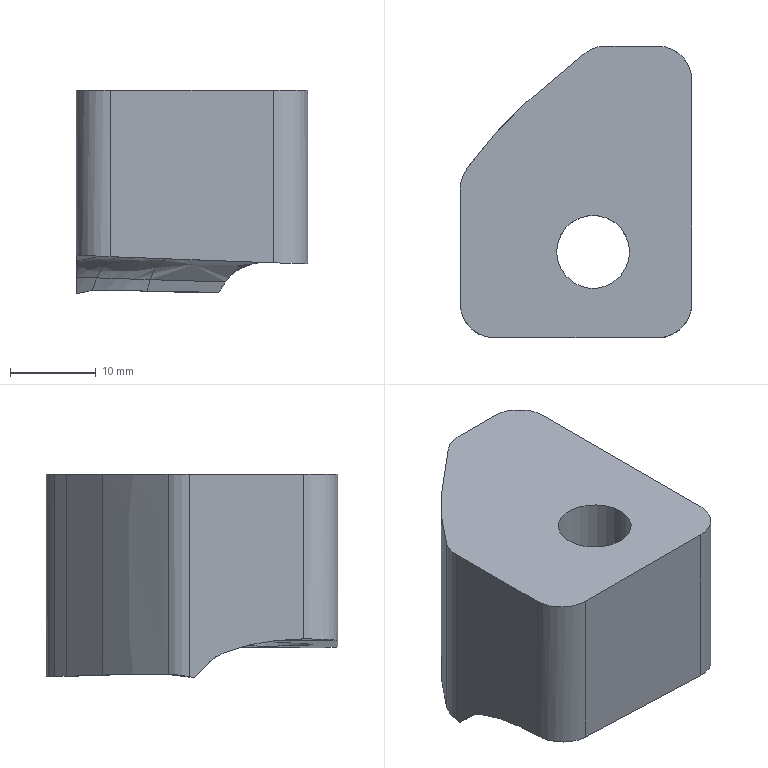Part | STEP file | gslz 2016.10.28-10_id1234_x_t | 1 solid | 27 faces | box 27 x 34 x 23.73 mm | volume 13778 mm3 | spline 10 | plane 7 | cylinder 7 | other 3 | commonest cylinder face diameters 8 x5 8.5 x1 14 x1